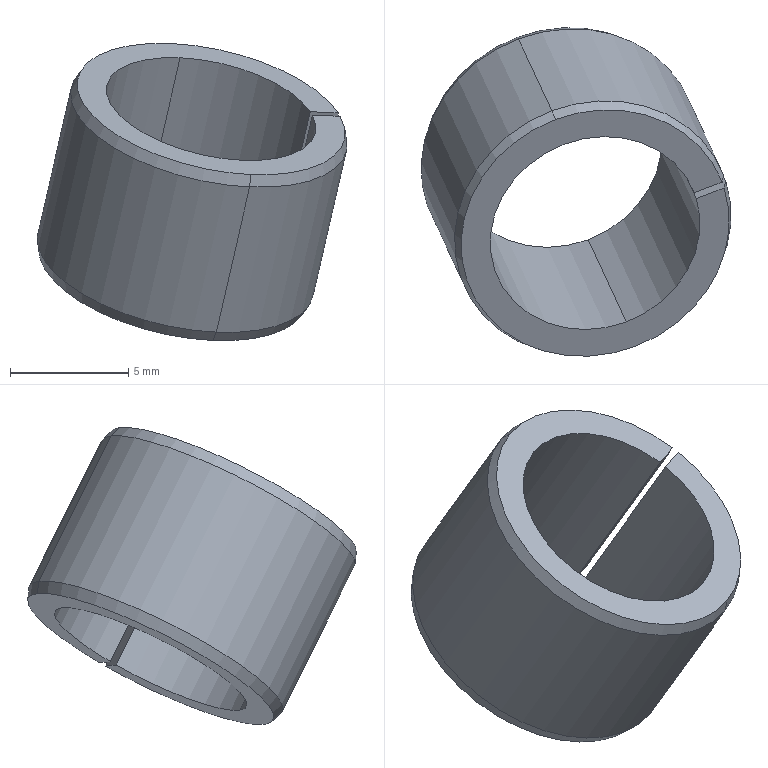Part | SolidWorks | features BaseBody 1 | 1 solid | 16 faces | box 13.105 x 13.906 x 12.577 mm | volume 373.199 mm3 | cylinder 6 | cone 6 | plane 4 | commonest cylinder face diameters 9.06 x3 11.94 x3
STEP:
#1=CARTESIAN_POINT('',(1952.49,-214.2,924.197));
#2=VERTEX_POINT('',#1);
#3=CARTESIAN_POINT('',(1949.865,-206.691,928.533));
#4=VERTEX_POINT('',#3);
#5=CARTESIAN_POINT('',(1951.178,-210.445,926.365));
#6=DIRECTION('',(-0.2015,0.436,-0.8771));
#7=DIRECTION('',(0.9447,0.3229,-0.05648));
#8=AXIS2_PLACEMENT_3D('',#5,#6,#7);
#9=CIRCLE('',#8,4.53);
#10=EDGE_CURVE('',#2,#4,#9,.T.);
#11=ORIENTED_EDGE('',*,*,#10,.F.);
#12=CARTESIAN_POINT('',(1950.879,-210.712,917.18));
#13=VERTEX_POINT('',#12);
#14=CARTESIAN_POINT('',(1952.523,-214.27,924.337));
#15=DIRECTION('',(-0.2015,0.436,-0.8771));
#16=VECTOR('',#15,1000.);
#17=LINE('',#14,#16);
#18=EDGE_CURVE('',#2,#13,#17,.T.);
#19=ORIENTED_EDGE('',*,*,#18,.T.);
#20=CARTESIAN_POINT('',(1948.254,-203.202,921.516));
#21=VERTEX_POINT('',#20);
#22=CARTESIAN_POINT('',(1949.566,-206.957,919.348));
#23=DIRECTION('',(0.2015,-0.436,0.8771));
#24=DIRECTION('',(0.9256,0.3778,-0.02479));
#25=AXIS2_PLACEMENT_3D('',#22,#23,#24);
#26=CIRCLE('',#25,4.53);
#27=EDGE_CURVE('',#21,#13,#26,.T.);
#28=ORIENTED_EDGE('',*,*,#27,.F.);
#29=CARTESIAN_POINT('',(1949.898,-206.76,928.673));
#30=DIRECTION('',(-0.2015,0.436,-0.8771));
#31=VECTOR('',#30,1000.);
#32=LINE('',#29,#31);
#33=EDGE_CURVE('',#4,#21,#32,.T.);
#34=ORIENTED_EDGE('',*,*,#33,.F.);
#35=EDGE_LOOP('',(#11,#19,#28,#34));
#36=FACE_OUTER_BOUND('',#35,.T.);
#37=CARTESIAN_POINT('',(1951.21,-210.515,926.505));
#38=DIRECTION('',(-0.2015,0.436,-0.8771));
#39=DIRECTION('',(-0.2897,0.8289,0.4786));
#40=AXIS2_PLACEMENT_3D('',#37,#38,#39);
#41=CYLINDRICAL_SURFACE('',#40,4.53);
#42=ADVANCED_FACE('',(#36),#41,.F.);
#43=CARTESIAN_POINT('',(1955.371,-208.734,926.253));
#44=VERTEX_POINT('',#43);
#45=CARTESIAN_POINT('',(1951.178,-210.445,926.365));
#46=DIRECTION('',(-0.2015,0.436,-0.8771));
#47=DIRECTION('',(0.9447,0.3229,-0.05648));
#48=AXIS2_PLACEMENT_3D('',#45,#46,#47);
#49=CIRCLE('',#48,4.53);
#50=EDGE_CURVE('',#4,#44,#49,.T.);
#51=ORIENTED_EDGE('',*,*,#50,.F.);
#52=ORIENTED_EDGE('',*,*,#33,.T.);
#53=CARTESIAN_POINT('',(1953.759,-205.246,919.236));
#54=VERTEX_POINT('',#53);
#55=CARTESIAN_POINT('',(1949.566,-206.957,919.348));
#56=DIRECTION('',(0.2015,-0.436,0.8771));
#57=DIRECTION('',(0.9256,0.3778,-0.02479));
#58=AXIS2_PLACEMENT_3D('',#55,#56,#57);
#59=CIRCLE('',#58,4.53);
#60=EDGE_CURVE('',#54,#21,#59,.T.);
#61=ORIENTED_EDGE('',*,*,#60,.F.);
#62=CARTESIAN_POINT('',(1955.371,-208.734,926.253));
#63=DIRECTION('',(-0.2015,0.436,-0.8771));
#64=VECTOR('',#63,1000.);
#65=LINE('',#62,#64);
#66=EDGE_CURVE('',#44,#54,#65,.T.);
#67=ORIENTED_EDGE('',*,*,#66,.F.);
#68=EDGE_LOOP('',(#51,#52,#61,#67));
#69=FACE_OUTER_BOUND('',#68,.T.);
#70=CARTESIAN_POINT('',(1951.21,-210.515,926.505));
#71=DIRECTION('',(-0.2015,0.436,-0.8771));
#72=DIRECTION('',(-0.2897,0.8289,0.4786));
#73=AXIS2_PLACEMENT_3D('',#70,#71,#72);
#74=CYLINDRICAL_SURFACE('',#73,4.53);
#75=ADVANCED_FACE('',(#69),#74,.F.);
#76=CARTESIAN_POINT('',(1947.889,-202.16,922.118));
#77=VERTEX_POINT('',#76);
#78=CARTESIAN_POINT('',(1954.936,-204.805,919.185));
#79=VERTEX_POINT('',#78);
#80=CARTESIAN_POINT('',(1949.566,-206.957,919.348));
#81=DIRECTION('',(-0.2015,0.436,-0.8771));
#82=DIRECTION('',(0.9429,0.329,-0.05305));
#83=AXIS2_PLACEMENT_3D('',#80,#81,#82);
#84=CIRCLE('',#83,5.788);
#85=EDGE_CURVE('',#77,#79,#84,.T.);
#86=ORIENTED_EDGE('',*,*,#85,.F.);
#87=CARTESIAN_POINT('',(1947.937,-202.227,922.644));
#88=VERTEX_POINT('',#87);
#89=CARTESIAN_POINT('',(1947.939,-202.23,922.666));
#90=DIRECTION('',(0.09022,-0.1262,0.9879));
#91=VECTOR('',#90,1000.);
#92=LINE('',#89,#91);
#93=EDGE_CURVE('',#77,#88,#92,.T.);
#94=ORIENTED_EDGE('',*,*,#93,.T.);
#95=CARTESIAN_POINT('',(1955.208,-204.959,919.616));
#96=VERTEX_POINT('',#95);
#97=CARTESIAN_POINT('',(1949.667,-207.175,919.787));
#98=DIRECTION('',(-0.2015,0.436,-0.8771));
#99=DIRECTION('',(0.9426,0.3296,-0.05267));
#100=AXIS2_PLACEMENT_3D('',#97,#98,#99);
#101=CIRCLE('',#100,5.97);
#102=EDGE_CURVE('',#88,#96,#101,.T.);
#103=ORIENTED_EDGE('',*,*,#102,.T.);
#104=CARTESIAN_POINT('',(1955.072,-204.882,919.4));
#105=DIRECTION('',(-0.5094,0.2898,-0.8103));
#106=VECTOR('',#105,1000.);
#107=LINE('',#104,#106);
#108=EDGE_CURVE('',#96,#79,#107,.T.);
#109=ORIENTED_EDGE('',*,*,#108,.T.);
#110=EDGE_LOOP('',(#86,#94,#103,#109));
#111=FACE_OUTER_BOUND('',#110,.T.);
#112=CARTESIAN_POINT('',(1949.671,-207.184,919.805));
#113=DIRECTION('',(0.2015,-0.436,0.8771));
#114=DIRECTION('',(0.2897,-0.8289,-0.4786));
#115=AXIS2_PLACEMENT_3D('',#112,#113,#114);
#116=CONICAL_SURFACE('',#115,5.978,0.3491);
#117=ADVANCED_FACE('',(#111),#116,.T.);
#118=ORIENTED_EDGE('',*,*,#93,.F.);
#119=CARTESIAN_POINT('',(1951.243,-211.755,916.578));
#120=VERTEX_POINT('',#119);
#121=CARTESIAN_POINT('',(1949.566,-206.957,919.348));
#122=DIRECTION('',(-0.2015,0.436,-0.8771));
#123=DIRECTION('',(0.9429,0.329,-0.05305));
#124=AXIS2_PLACEMENT_3D('',#121,#122,#123);
#125=CIRCLE('',#124,5.788);
#126=EDGE_CURVE('',#120,#77,#125,.T.);
#127=ORIENTED_EDGE('',*,*,#126,.F.);
#128=CARTESIAN_POINT('',(1951.397,-212.123,916.93));
#129=VERTEX_POINT('',#128);
#130=CARTESIAN_POINT('',(1951.403,-212.139,916.945));
#131=DIRECTION('',(0.2884,-0.6932,0.6605));
#132=VECTOR('',#131,1000.);
#133=LINE('',#130,#132);
#134=EDGE_CURVE('',#120,#129,#133,.T.);
#135=ORIENTED_EDGE('',*,*,#134,.T.);
#136=CARTESIAN_POINT('',(1949.667,-207.175,919.787));
#137=DIRECTION('',(-0.2015,0.436,-0.8771));
#138=DIRECTION('',(0.9426,0.3296,-0.05267));
#139=AXIS2_PLACEMENT_3D('',#136,#137,#138);
#140=CIRCLE('',#139,5.97);
#141=EDGE_CURVE('',#129,#88,#140,.T.);
#142=ORIENTED_EDGE('',*,*,#141,.T.);
#143=EDGE_LOOP('',(#118,#127,#135,#142));
#144=FACE_OUTER_BOUND('',#143,.T.);
#145=CARTESIAN_POINT('',(1949.671,-207.184,919.805));
#146=DIRECTION('',(0.2015,-0.436,0.8771));
#147=DIRECTION('',(0.2897,-0.8289,-0.4786));
#148=AXIS2_PLACEMENT_3D('',#145,#146,#147);
#149=CONICAL_SURFACE('',#148,5.978,0.3491);
#150=ADVANCED_FACE('',(#144),#149,.T.);
#151=CARTESIAN_POINT('',(1952.807,-215.176,923.069));
#152=VERTEX_POINT('',#151);
#153=CARTESIAN_POINT('',(1956.705,-208.26,925.612));
#154=VERTEX_POINT('',#153);
#155=CARTESIAN_POINT('',(1951.077,-210.227,925.927));
#156=DIRECTION('',(0.2015,-0.436,0.8771));
#157=DIRECTION('',(0.9281,0.3713,-0.02862));
#158=AXIS2_PLACEMENT_3D('',#155,#156,#157);
#159=CIRCLE('',#158,5.97);
#160=EDGE_CURVE('',#152,#154,#159,.T.);
#161=ORIENTED_EDGE('',*,*,#160,.F.);
#162=CARTESIAN_POINT('',(1952.835,-215.237,923.192));
#163=DIRECTION('',(-0.2015,0.436,-0.8771));
#164=VECTOR('',#163,1000.);
#165=LINE('',#162,#164);
#166=EDGE_CURVE('',#152,#129,#165,.T.);
#167=ORIENTED_EDGE('',*,*,#166,.T.);
#168=CARTESIAN_POINT('',(1955.294,-205.207,919.472));
#169=VERTEX_POINT('',#168);
#170=CARTESIAN_POINT('',(1949.667,-207.175,919.787));
#171=DIRECTION('',(-0.2015,0.436,-0.8771));
#172=DIRECTION('',(0.9426,0.3296,-0.05267));
#173=AXIS2_PLACEMENT_3D('',#170,#171,#172);
#174=CIRCLE('',#173,5.97);
#175=EDGE_CURVE('',#169,#129,#174,.T.);
#176=ORIENTED_EDGE('',*,*,#175,.F.);
#177=CARTESIAN_POINT('',(1956.705,-208.26,925.612));
#178=DIRECTION('',(-0.2015,0.436,-0.8771));
#179=VECTOR('',#178,1000.);
#180=LINE('',#177,#179);
#181=EDGE_CURVE('',#154,#169,#180,.T.);
#182=ORIENTED_EDGE('',*,*,#181,.F.);
#183=EDGE_LOOP('',(#161,#167,#176,#182));
#184=FACE_OUTER_BOUND('',#183,.T.);
#185=CARTESIAN_POINT('',(1951.105,-210.288,926.049));
#186=DIRECTION('',(-0.2015,0.436,-0.8771));
#187=DIRECTION('',(-0.2897,0.8289,0.4786));
#188=AXIS2_PLACEMENT_3D('',#185,#186,#187);
#189=CYLINDRICAL_SURFACE('',#188,5.97);
#190=ADVANCED_FACE('',(#184),#189,.T.);
#191=ORIENTED_EDGE('',*,*,#166,.F.);
#192=CARTESIAN_POINT('',(1949.347,-205.279,928.784));
#193=VERTEX_POINT('',#192);
#194=CARTESIAN_POINT('',(1951.077,-210.227,925.927));
#195=DIRECTION('',(0.2015,-0.436,0.8771));
#196=DIRECTION('',(0.9281,0.3713,-0.02862));
#197=AXIS2_PLACEMENT_3D('',#194,#195,#196);
#198=CIRCLE('',#197,5.97);
#199=EDGE_CURVE('',#193,#152,#198,.T.);
#200=ORIENTED_EDGE('',*,*,#199,.F.);
#201=CARTESIAN_POINT('',(1949.376,-205.34,928.907));
#202=DIRECTION('',(-0.2015,0.436,-0.8771));
#203=VECTOR('',#202,1000.);
#204=LINE('',#201,#203);
#205=EDGE_CURVE('',#193,#88,#204,.T.);
#206=ORIENTED_EDGE('',*,*,#205,.T.);
#207=ORIENTED_EDGE('',*,*,#141,.F.);
#208=EDGE_LOOP('',(#191,#200,#206,#207));
#209=FACE_OUTER_BOUND('',#208,.T.);
#210=CARTESIAN_POINT('',(1951.105,-210.288,926.049));
#211=DIRECTION('',(-0.2015,0.436,-0.8771));
#212=DIRECTION('',(-0.2897,0.8289,0.4786));
#213=AXIS2_PLACEMENT_3D('',#210,#211,#212);
#214=CYLINDRICAL_SURFACE('',#213,5.97);
#215=ADVANCED_FACE('',(#209),#214,.T.);
#216=CARTESIAN_POINT('',(1952.855,-215.243,923.595));
#217=VERTEX_POINT('',#216);
#218=CARTESIAN_POINT('',(1956.635,-208.541,926.058));
#219=VERTEX_POINT('',#218);
#220=CARTESIAN_POINT('',(1951.178,-210.445,926.365));
#221=DIRECTION('',(0.2015,-0.436,0.8771));
#222=DIRECTION('',(0.9278,0.3719,-0.02824));
#223=AXIS2_PLACEMENT_3D('',#220,#221,#222);
#224=CIRCLE('',#223,5.788);
#225=EDGE_CURVE('',#217,#219,#224,.T.);
#226=ORIENTED_EDGE('',*,*,#225,.F.);
#227=CARTESIAN_POINT('',(1952.857,-215.246,923.617));
#228=DIRECTION('',(-0.09022,0.1262,-0.9879));
#229=VECTOR('',#228,1000.);
#230=LINE('',#227,#229);
#231=EDGE_CURVE('',#217,#152,#230,.T.);
#232=ORIENTED_EDGE('',*,*,#231,.T.);
#233=ORIENTED_EDGE('',*,*,#160,.T.);
#234=CARTESIAN_POINT('',(1956.67,-208.401,925.835));
#235=DIRECTION('',(-0.1308,-0.5296,0.8381));
#236=VECTOR('',#235,1000.);
#237=LINE('',#234,#236);
#238=EDGE_CURVE('',#154,#219,#237,.T.);
#239=ORIENTED_EDGE('',*,*,#238,.T.);
#240=EDGE_LOOP('',(#226,#232,#233,#239));
#241=FACE_OUTER_BOUND('',#240,.T.);
#242=CARTESIAN_POINT('',(1951.182,-210.454,926.384));
#243=DIRECTION('',(-0.2015,0.436,-0.8771));
#244=DIRECTION('',(-0.2897,0.8289,0.4786));
#245=AXIS2_PLACEMENT_3D('',#242,#243,#244);
#246=CONICAL_SURFACE('',#245,5.78,0.3491);
#247=ADVANCED_FACE('',(#241),#246,.T.);
#248=ORIENTED_EDGE('',*,*,#231,.F.);
#249=CARTESIAN_POINT('',(1949.501,-205.648,929.135));
#250=VERTEX_POINT('',#249);
#251=CARTESIAN_POINT('',(1951.178,-210.445,926.365));
#252=DIRECTION('',(0.2015,-0.436,0.8771));
#253=DIRECTION('',(0.9278,0.3719,-0.02824));
#254=AXIS2_PLACEMENT_3D('',#251,#252,#253);
#255=CIRCLE('',#254,5.788);
#256=EDGE_CURVE('',#250,#217,#255,.T.);
#257=ORIENTED_EDGE('',*,*,#256,.F.);
#258=CARTESIAN_POINT('',(1949.507,-205.663,929.15));
#259=DIRECTION('',(-0.2884,0.6932,-0.6605));
#260=VECTOR('',#259,1000.);
#261=LINE('',#258,#260);
#262=EDGE_CURVE('',#250,#193,#261,.T.);
#263=ORIENTED_EDGE('',*,*,#262,.T.);
#264=ORIENTED_EDGE('',*,*,#199,.T.);
#265=EDGE_LOOP('',(#248,#257,#263,#264));
#266=FACE_OUTER_BOUND('',#265,.T.);
#267=CARTESIAN_POINT('',(1951.182,-210.454,926.384));
#268=DIRECTION('',(-0.2015,0.436,-0.8771));
#269=DIRECTION('',(-0.2897,0.8289,0.4786));
#270=AXIS2_PLACEMENT_3D('',#267,#268,#269);
#271=CONICAL_SURFACE('',#270,5.78,0.3491);
#272=ADVANCED_FACE('',(#266),#271,.T.);
#273=CARTESIAN_POINT('',(1956.548,-208.293,926.202));
#274=VERTEX_POINT('',#273);
#275=CARTESIAN_POINT('',(1951.178,-210.445,926.365));
#276=DIRECTION('',(0.2015,-0.436,0.8771));
#277=DIRECTION('',(0.9278,0.3719,-0.02824));
#278=AXIS2_PLACEMENT_3D('',#275,#276,#277);
#279=CIRCLE('',#278,5.788);
#280=EDGE_CURVE('',#274,#250,#279,.T.);
#281=ORIENTED_EDGE('',*,*,#280,.T.);
#282=ORIENTED_EDGE('',*,*,#256,.T.);
#283=ORIENTED_EDGE('',*,*,#225,.T.);
#284=CARTESIAN_POINT('',(1955.458,-208.983,926.109));
#285=VERTEX_POINT('',#284);
#286=CARTESIAN_POINT('',(1956.635,-208.541,926.058));
#287=DIRECTION('',(-0.9357,-0.3505,0.04066));
#288=VECTOR('',#287,1000.);
#289=LINE('',#286,#288);
#290=EDGE_CURVE('',#219,#285,#289,.T.);
#291=ORIENTED_EDGE('',*,*,#290,.T.);
#292=CARTESIAN_POINT('',(1951.178,-210.445,926.365));
#293=DIRECTION('',(-0.2015,0.436,-0.8771));
#294=DIRECTION('',(0.9447,0.3229,-0.05648));
#295=AXIS2_PLACEMENT_3D('',#292,#293,#294);
#296=CIRCLE('',#295,4.53);
#297=EDGE_CURVE('',#285,#2,#296,.T.);
#298=ORIENTED_EDGE('',*,*,#297,.T.);
#299=ORIENTED_EDGE('',*,*,#10,.T.);
#300=ORIENTED_EDGE('',*,*,#50,.T.);
#301=CARTESIAN_POINT('',(1956.548,-208.293,926.202));
#302=DIRECTION('',(-0.9357,-0.3505,0.04066));
#303=VECTOR('',#302,1000.);
#304=LINE('',#301,#303);
#305=EDGE_CURVE('',#274,#44,#304,.T.);
#306=ORIENTED_EDGE('',*,*,#305,.F.);
#307=EDGE_LOOP('',(#281,#282,#283,#291,#298,#299,#300,#306));
#308=FACE_OUTER_BOUND('',#307,.T.);
#309=CARTESIAN_POINT('',(1943.797,-207.566,929.492));
#310=DIRECTION('',(0.2015,-0.436,0.8771));
#311=DIRECTION('',(0.2897,-0.8289,-0.4786));
#312=AXIS2_PLACEMENT_3D('',#309,#310,#311);
#313=PLANE('',#312);
#314=ADVANCED_FACE('',(#308),#313,.T.);
#315=ORIENTED_EDGE('',*,*,#66,.T.);
#316=CARTESIAN_POINT('',(1954.936,-204.805,919.185));
#317=DIRECTION('',(-0.9357,-0.3505,0.04066));
#318=VECTOR('',#317,1000.);
#319=LINE('',#316,#318);
#320=EDGE_CURVE('',#79,#54,#319,.T.);
#321=ORIENTED_EDGE('',*,*,#320,.F.);
#322=ORIENTED_EDGE('',*,*,#108,.F.);
#323=CARTESIAN_POINT('',(1956.618,-208.011,925.756));
#324=VERTEX_POINT('',#323);
#325=CARTESIAN_POINT('',(1956.618,-208.011,925.756));
#326=DIRECTION('',(-0.2015,0.436,-0.8771));
#327=VECTOR('',#326,1000.);
#328=LINE('',#325,#327);
#329=EDGE_CURVE('',#324,#96,#328,.T.);
#330=ORIENTED_EDGE('',*,*,#329,.F.);
#331=CARTESIAN_POINT('',(1956.583,-208.152,925.979));
#332=DIRECTION('',(-0.1308,-0.5296,0.8381));
#333=VECTOR('',#332,1000.);
#334=LINE('',#331,#333);
#335=EDGE_CURVE('',#324,#274,#334,.T.);
#336=ORIENTED_EDGE('',*,*,#335,.T.);
#337=ORIENTED_EDGE('',*,*,#305,.T.);
#338=EDGE_LOOP('',(#315,#321,#322,#330,#336,#337));
#339=FACE_OUTER_BOUND('',#338,.T.);
#340=CARTESIAN_POINT('',(1955.376,-208.814,926.394));
#341=DIRECTION('',(0.2897,-0.8289,-0.4786));
#342=DIRECTION('',(-0.2015,0.436,-0.8771));
#343=AXIS2_PLACEMENT_3D('',#340,#341,#342);
#344=PLANE('',#343);
#345=ADVANCED_FACE('',(#339),#344,.T.);
#346=ORIENTED_EDGE('',*,*,#262,.F.);
#347=ORIENTED_EDGE('',*,*,#280,.F.);
#348=ORIENTED_EDGE('',*,*,#335,.F.);
#349=CARTESIAN_POINT('',(1951.077,-210.227,925.927));
#350=DIRECTION('',(0.2015,-0.436,0.8771));
#351=DIRECTION('',(0.9281,0.3713,-0.02862));
#352=AXIS2_PLACEMENT_3D('',#349,#350,#351);
#353=CIRCLE('',#352,5.97);
#354=EDGE_CURVE('',#324,#193,#353,.T.);
#355=ORIENTED_EDGE('',*,*,#354,.T.);
#356=EDGE_LOOP('',(#346,#347,#348,#355));
#357=FACE_OUTER_BOUND('',#356,.T.);
#358=CARTESIAN_POINT('',(1951.182,-210.454,926.384));
#359=DIRECTION('',(-0.2015,0.436,-0.8771));
#360=DIRECTION('',(-0.2897,0.8289,0.4786));
#361=AXIS2_PLACEMENT_3D('',#358,#359,#360);
#362=CONICAL_SURFACE('',#361,5.78,0.3491);
#363=ADVANCED_FACE('',(#357),#362,.T.);
#364=ORIENTED_EDGE('',*,*,#205,.F.);
#365=ORIENTED_EDGE('',*,*,#354,.F.);
#366=ORIENTED_EDGE('',*,*,#329,.T.);
#367=ORIENTED_EDGE('',*,*,#102,.F.);
#368=EDGE_LOOP('',(#364,#365,#366,#367));
#369=FACE_OUTER_BOUND('',#368,.T.);
#370=CARTESIAN_POINT('',(1951.105,-210.288,926.049));
#371=DIRECTION('',(-0.2015,0.436,-0.8771));
#372=DIRECTION('',(-0.2897,0.8289,0.4786));
#373=AXIS2_PLACEMENT_3D('',#370,#371,#372);
#374=CYLINDRICAL_SURFACE('',#373,5.97);
#375=ADVANCED_FACE('',(#369),#374,.T.);
#376=ORIENTED_EDGE('',*,*,#134,.F.);
#377=CARTESIAN_POINT('',(1955.023,-205.053,919.041));
#378=VERTEX_POINT('',#377);
#379=CARTESIAN_POINT('',(1949.566,-206.957,919.348));
#380=DIRECTION('',(-0.2015,0.436,-0.8771));
#381=DIRECTION('',(0.9429,0.329,-0.05305));
#382=AXIS2_PLACEMENT_3D('',#379,#380,#381);
#383=CIRCLE('',#382,5.788);
#384=EDGE_CURVE('',#378,#120,#383,.T.);
#385=ORIENTED_EDGE('',*,*,#384,.F.);
#386=CARTESIAN_POINT('',(1955.159,-205.13,919.257));
#387=DIRECTION('',(-0.5094,0.2898,-0.8103));
#388=VECTOR('',#387,1000.);
#389=LINE('',#386,#388);
#390=EDGE_CURVE('',#169,#378,#389,.T.);
#391=ORIENTED_EDGE('',*,*,#390,.F.);
#392=ORIENTED_EDGE('',*,*,#175,.T.);
#393=EDGE_LOOP('',(#376,#385,#391,#392));
#394=FACE_OUTER_BOUND('',#393,.T.);
#395=CARTESIAN_POINT('',(1949.671,-207.184,919.805));
#396=DIRECTION('',(0.2015,-0.436,0.8771));
#397=DIRECTION('',(0.2897,-0.8289,-0.4786));
#398=AXIS2_PLACEMENT_3D('',#395,#396,#397);
#399=CONICAL_SURFACE('',#398,5.978,0.3491);
#400=ADVANCED_FACE('',(#394),#399,.T.);
#401=ORIENTED_EDGE('',*,*,#238,.F.);
#402=ORIENTED_EDGE('',*,*,#181,.T.);
#403=ORIENTED_EDGE('',*,*,#390,.T.);
#404=CARTESIAN_POINT('',(1953.846,-205.494,919.092));
#405=VERTEX_POINT('',#404);
#406=CARTESIAN_POINT('',(1955.023,-205.053,919.041));
#407=DIRECTION('',(-0.9357,-0.3505,0.04066));
#408=VECTOR('',#407,1000.);
#409=LINE('',#406,#408);
#410=EDGE_CURVE('',#378,#405,#409,.T.);
#411=ORIENTED_EDGE('',*,*,#410,.T.);
#412=CARTESIAN_POINT('',(1955.458,-208.983,926.109));
#413=DIRECTION('',(-0.2015,0.436,-0.8771));
#414=VECTOR('',#413,1000.);
#415=LINE('',#412,#414);
#416=EDGE_CURVE('',#285,#405,#415,.T.);
#417=ORIENTED_EDGE('',*,*,#416,.F.);
#418=ORIENTED_EDGE('',*,*,#290,.F.);
#419=EDGE_LOOP('',(#401,#402,#403,#411,#417,#418));
#420=FACE_OUTER_BOUND('',#419,.T.);
#421=CARTESIAN_POINT('',(1956.865,-208.537,926.19));
#422=DIRECTION('',(-0.2897,0.8289,0.4786));
#423=DIRECTION('',(-0.2015,0.436,-0.8771));
#424=AXIS2_PLACEMENT_3D('',#421,#422,#423);
#425=PLANE('',#424);
#426=ADVANCED_FACE('',(#420),#425,.T.);
#427=ORIENTED_EDGE('',*,*,#18,.F.);
#428=ORIENTED_EDGE('',*,*,#297,.F.);
#429=ORIENTED_EDGE('',*,*,#416,.T.);
#430=CARTESIAN_POINT('',(1949.566,-206.957,919.348));
#431=DIRECTION('',(0.2015,-0.436,0.8771));
#432=DIRECTION('',(0.9256,0.3778,-0.02479));
#433=AXIS2_PLACEMENT_3D('',#430,#431,#432);
#434=CIRCLE('',#433,4.53);
#435=EDGE_CURVE('',#13,#405,#434,.T.);
#436=ORIENTED_EDGE('',*,*,#435,.F.);
#437=EDGE_LOOP('',(#427,#428,#429,#436));
#438=FACE_OUTER_BOUND('',#437,.T.);
#439=CARTESIAN_POINT('',(1951.21,-210.515,926.505));
#440=DIRECTION('',(-0.2015,0.436,-0.8771));
#441=DIRECTION('',(-0.2897,0.8289,0.4786));
#442=AXIS2_PLACEMENT_3D('',#439,#440,#441);
#443=CYLINDRICAL_SURFACE('',#442,4.53);
#444=ADVANCED_FACE('',(#438),#443,.F.);
#445=ORIENTED_EDGE('',*,*,#60,.T.);
#446=ORIENTED_EDGE('',*,*,#27,.T.);
#447=ORIENTED_EDGE('',*,*,#435,.T.);
#448=ORIENTED_EDGE('',*,*,#410,.F.);
#449=ORIENTED_EDGE('',*,*,#384,.T.);
#450=ORIENTED_EDGE('',*,*,#126,.T.);
#451=ORIENTED_EDGE('',*,*,#85,.T.);
#452=ORIENTED_EDGE('',*,*,#320,.T.);
#453=EDGE_LOOP('',(#445,#446,#447,#448,#449,#450,#451,#452));
#454=FACE_OUTER_BOUND('',#453,.T.);
#455=CARTESIAN_POINT('',(1942.185,-204.078,922.475));
#456=DIRECTION('',(-0.2015,0.436,-0.8771));
#457=DIRECTION('',(0.9357,0.3505,-0.04066));
#458=AXIS2_PLACEMENT_3D('',#455,#456,#457);
#459=PLANE('',#458);
#460=ADVANCED_FACE('',(#454),#459,.T.);
#461=CLOSED_SHELL('',(#42,#75,#117,#150,#190,#215,#247,#272,#314,#345,#363,#375,#400,#426,#444,#460));
#462=MANIFOLD_SOLID_BREP('',#461);
#463=CARTESIAN_POINT('',(0.,0.,0.));
#464=DIRECTION('',(0.,0.,1.));
#465=DIRECTION('',(1.,0.,0.));
#466=AXIS2_PLACEMENT_3D('',#463,#464,#465);
#467=(LENGTH_UNIT()NAMED_UNIT(*)SI_UNIT(.MILLI.,.METRE.));
#468=UNCERTAINTY_MEASURE_WITH_UNIT(LENGTH_MEASURE(0.00001),#467,'','');
#469=(NAMED_UNIT(*)PLANE_ANGLE_UNIT()SI_UNIT($,.RADIAN.));
#470=(NAMED_UNIT(*)SI_UNIT($,.STERADIAN.)SOLID_ANGLE_UNIT());
#471=(GEOMETRIC_REPRESENTATION_CONTEXT(3)GLOBAL_UNCERTAINTY_ASSIGNED_CONTEXT((#468))GLOBAL_UNIT_ASSIGNED_CONTEXT((#467,#469,#470))REPRESENTATION_CONTEXT('',''));
#472=ADVANCED_BREP_SHAPE_REPRESENTATION('',(#462,#466),#471);